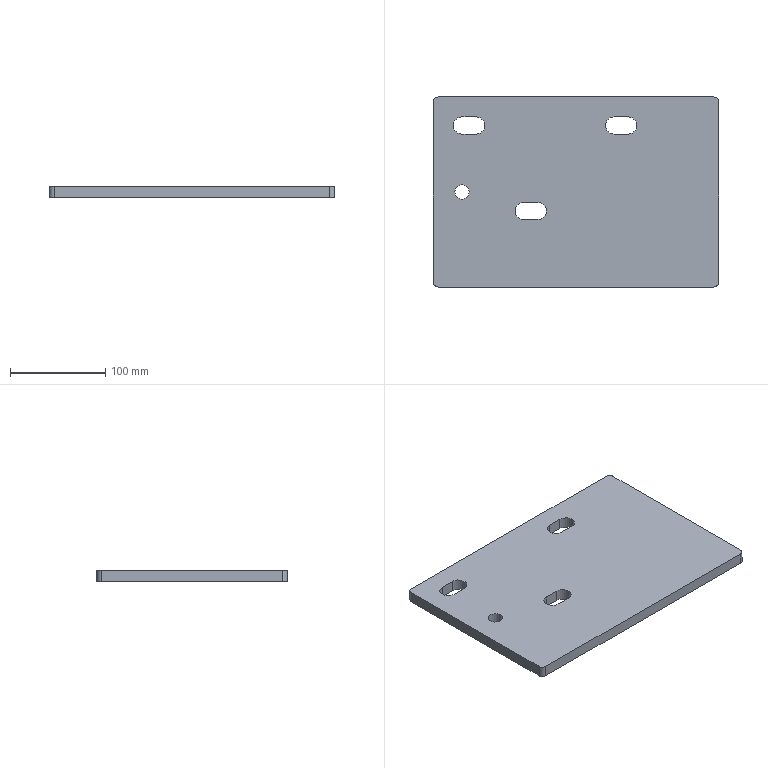Part | STEP file | Sheet20 | 1 solid | 23 faces | box 300 x 200 x 12 mm | volume 698741 mm3 | plane 12 | cylinder 11 | commonest cylinder face diameters 18 x6 10 x4 15 x1